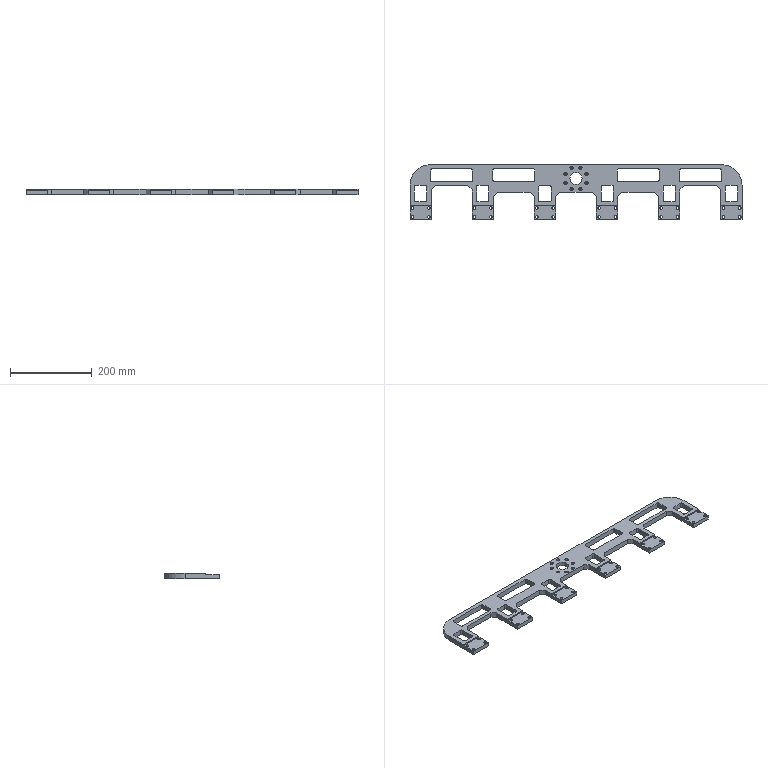NC program | NX | posted with a generic post | part box 813.6 x 134 x 13 mm
Lines 5528 to 6062 of 6062:
(PLANAR_MILL_COPY_1_COPY_1 , TOOL : D6A45)
N11006 T07 M6
N11008 G54
N11010 G17 G0 G90 X360.312 Y-40.242 S9500 M3
N11012 G43 Z30. H7
N11014 Z0.
N11016 G94 G1 Z-1. F1400.
N11018 X359.934 Y-41.05
N11020 G3 X360.8 Y-41.55 R1.
N11022 X363.15 Y-39.2 R2.35
N11024 X360.8 Y-41.55 R-2.35
N11026 X361.666 Y-41.05 R1.
N11028 G1 X361.288 Y-40.242
N11030 Z0.
N11032 G0 Z30.
N11034 X360.312 Y-62.242
N11036 Z0.
N11038 G1 Z-1.
N11040 X359.934 Y-63.05
N11042 G3 X360.8 Y-63.55 R1.
N11044 X363.15 Y-61.2 R2.35
N11046 X360.8 Y-63.55 R-2.35
N11048 X361.666 Y-63.05 R1.
N11050 G1 X361.288 Y-62.242
N11052 Z0.
N11054 G0 Z30.
N11056 X400.312
N11058 Z0.
N11060 G1 Z-1.
N11062 X399.934 Y-63.05
N11064 G3 X400.8 Y-63.55 R1.
N11066 X403.15 Y-61.2 R2.35
N11068 X400.8 Y-63.55 R-2.35
N11070 X401.666 Y-63.05 R1.
N11072 G1 X401.288 Y-62.242
N11074 Z0.
N11076 G0 Z30.
N11078 X401.842 Y-39.688
N11080 Z0.
N11082 G1 Z-1.
N11084 X402.65 Y-40.066
N11086 G3 X403.15 Y-39.2 R1.
N11088 X400.8 Y-36.85 R2.35
N11090 X403.15 Y-39.2 R-2.35
N11092 X402.65 Y-38.334 R1.
N11094 G1 X401.842 Y-38.712
N11096 Z0.
N11098 G0 Z30.
N11100 X393.7 Y-5.27
N11102 Z0.
N11104 G1 Z-1.
N11106 X394.4 Y-4.866
N11108 G3 X394.9 Y-4. R1.
N11110 G1 Y13.
N11112 G3 X392.8 Y15.1 R2.1
N11114 G1 X368.8
N11116 G3 X366.7 Y13. R2.1
N11118 G1 Y-21.
N11120 G3 X368.8 Y-23.1 R2.1
N11122 G1 X392.8
N11124 G3 X394.9 Y-21. R2.1
N11126 G1 Y-4.
N11128 G3 X394.4 Y-3.134 R1.
N11130 G1 X393.7 Y-2.73
N11132 Z0.
N11134 G0 Z30.
N11136 X306.07 Y54.9
N11138 Z0.
N11140 G1 Z-1.
N11142 X305.666 Y55.6
N11144 G3 X304.8 Y56.1 R1.
N11146 G1 X256.8
N11148 G3 X254.7 Y54. R2.1
N11150 G1 Y28.
N11152 G3 X256.8 Y25.9 R2.1
N11154 G1 X352.8
N11156 G3 X354.9 Y28. R2.1
N11158 G1 Y54.
N11160 G3 X352.8 Y56.1 R2.1
N11162 G1 X304.8
N11164 G3 X303.934 Y55.6 R1.
N11166 G1 X303.53 Y54.9
N11168 Z0.
N11170 G0 Z30.
N11172 X247.912 Y-40.242
N11174 Z0.
N11176 G1 Z-1.
N11178 X247.534 Y-41.05
N11180 G3 X248.4 Y-41.55 R1.
N11182 X250.75 Y-39.2 R2.35
N11184 X248.4 Y-41.55 R-2.35
N11186 X249.266 Y-41.05 R1.
N11188 G1 X248.888 Y-40.242
N11190 Z0.
N11192 G0 Z30.
N11194 X247.912 Y-62.242
N11196 Z0.
N11198 G1 Z-1.
N11200 X247.534 Y-63.05
N11202 G3 X248.4 Y-63.55 R1.
N11204 X250.75 Y-61.2 R2.35
N11206 X248.4 Y-63.55 R-2.35
N11208 X249.266 Y-63.05 R1.
N11210 G1 X248.888 Y-62.242
N11212 Z0.
N11214 G0 Z30.
N11216 X207.912
N11218 Z0.
N11220 G1 Z-1.
N11222 X207.534 Y-63.05
N11224 G3 X208.4 Y-63.55 R1.
N11226 X210.75 Y-61.2 R2.35
N11228 X208.4 Y-63.55 R-2.35
N11230 X209.266 Y-63.05 R1.
N11232 G1 X208.888 Y-62.242
N11234 Z0.
N11236 G0 Z30.
N11238 X207.912 Y-40.242
N11240 Z0.
N11242 G1 Z-1.
N11244 X207.534 Y-41.05
N11246 G3 X208.4 Y-41.55 R1.
N11248 X210.75 Y-39.2 R2.35
N11250 X208.4 Y-41.55 R-2.35
N11252 X209.266 Y-41.05 R1.
N11254 G1 X208.888 Y-40.242
N11256 Z0.
N11258 G0 Z30.
N11260 X215.5 Y-2.73
N11262 Z0.
N11264 G1 Z-1.
N11266 X214.8 Y-3.134
N11268 G3 X214.3 Y-4. R1.
N11270 G1 Y-21.
N11272 G3 X216.4 Y-23.1 R2.1
N11274 G1 X240.4
N11276 G3 X242.5 Y-21. R2.1
N11278 G1 Y13.
N11280 G3 X240.4 Y15.1 R2.1
N11282 G1 X216.4
N11284 G3 X214.3 Y13. R2.1
N11286 G1 Y-4.
N11288 G3 X214.8 Y-4.866 R1.
N11290 G1 X215.5 Y-5.27
N11292 Z0.
N11294 G0 Z30.
N11296 X153.67 Y54.9
N11298 Z0.
N11300 G1 Z-1.
N11302 X153.266 Y55.6
N11304 G3 X152.4 Y56.1 R1.
N11306 G1 X104.4
N11308 G3 X102.3 Y54. R2.1
N11310 G1 Y28.
N11312 G3 X104.4 Y25.9 R2.1
N11314 G1 X200.4
N11316 G3 X202.5 Y28. R2.1
N11318 G1 Y54.
N11320 G3 X200.4 Y56.1 R2.1
N11322 G1 X152.4
N11324 G3 X151.534 Y55.6 R1.
N11326 G1 X151.13 Y54.9
N11328 Z0.
N11330 G0 Z30.
N11332 X88.9 Y-5.27
N11334 Z0.
N11336 G1 Z-1.
N11338 X89.6 Y-4.866
N11340 G3 X90.1 Y-4. R1.
N11342 G1 Y13.
N11344 G3 X88. Y15.1 R2.1
N11346 G1 X64.
N11348 G3 X61.9 Y13. R2.1
N11350 G1 Y-21.
N11352 G3 X64. Y-23.1 R2.1
N11354 G1 X88.
N11356 G3 X90.1 Y-21. R2.1
N11358 G1 Y-4.
N11360 G3 X89.6 Y-3.134 R1.
N11362 G1 X88.9 Y-2.73
N11364 Z0.
N11366 G0 Z30.
N11368 X95.512 Y-40.242
N11370 Z0.
N11372 G1 Z-1.
N11374 X95.134 Y-41.05
N11376 G3 X96. Y-41.55 R1.
N11378 X98.35 Y-39.2 R2.35
N11380 X96. Y-41.55 R-2.35
N11382 X96.866 Y-41.05 R1.
N11384 G1 X96.488 Y-40.242
N11386 Z0.
N11388 G0 Z30.
N11390 X95.512 Y-62.242
N11392 Z0.
N11394 G1 Z-1.
N11396 X95.134 Y-63.05
N11398 G3 X96. Y-63.55 R1.
N11400 X98.35 Y-61.2 R2.35
N11402 X96. Y-63.55 R-2.35
N11404 X96.866 Y-63.05 R1.
N11406 G1 X96.488 Y-62.242
N11408 Z0.
N11410 G0 Z30.
N11412 X55.512
N11414 Z0.
N11416 G1 Z-1.
N11418 X55.134 Y-63.05
N11420 G3 X56. Y-63.55 R1.
N11422 X58.35 Y-61.2 R2.35
N11424 X56. Y-63.55 R-2.35
N11426 X56.866 Y-63.05 R1.
N11428 G1 X56.488 Y-62.242
N11430 Z0.
N11432 G0 Z30.
N11434 X55.512 Y-40.242
N11436 Z0.
N11438 G1 Z-1.
N11440 X55.134 Y-41.05
N11442 G3 X56. Y-41.55 R1.
N11444 X58.35 Y-39.2 R2.35
N11446 X56. Y-41.55 R-2.35
N11448 X56.866 Y-41.05 R1.
N11450 G1 X56.488 Y-40.242
N11452 Z0.
N11454 G0 Z30.
N11456 X1.287 Y62.021
N11458 Z0.
N11460 G1 Z-1.
N11462 X0.866 Y62.75
N11464 G3 X0. Y63.25 R1.
N11466 X-30.25 Y33. R30.25
N11468 X0. Y63.25 R-30.25
N11470 X-0.866 Y62.75 R1.
N11472 G1 X-1.287 Y62.021
N11474 Z0.
N11476 G0 Z30.
N11478 X-1.27 Y69.1
N11480 Z0.
N11482 G1 Z-1.
N11484 X-0.866 Y68.4
N11486 G3 X0. Y67.9 R1.
N11488 G1 X356.8
N11490 G2 X407.7 Y17. R50.9
N11492 G1 Y-66.9
N11494 G2 X406.7 Y-67.9 R1.
N11496 G1 X354.9
N11498 G2 X353.9 Y-66.9 R1.
N11500 G1 Y4.627
N11502 X344.427 Y14.1
N11504 X265.173
N11506 X255.7 Y4.627
N11508 Y-66.9
N11510 G2 X254.7 Y-67.9 R1.
N11512 G1 X202.5
N11514 G2 X201.5 Y-66.9 R1.
N11516 G1 Y-11.323
N11518 X192.027 Y-1.85
N11520 X112.773
N11522 X103.3 Y-11.323
N11524 Y-66.9
N11526 G2 X102.3 Y-67.9 R1.
N11528 G1 X50.1
N11530 G2 X49.1 Y-66.9 R1.
N11532 G1 Y-11.323
N11534 X39.627 Y-1.85
N11536 X-39.627
N11538 X-49.1 Y-11.323
N11540 Y-66.9
N11542 G2 X-50.1 Y-67.9 R1.
N11544 G1 X-102.3
N11546 G2 X-103.3 Y-66.9 R1.
N11548 G1 Y-11.323
N11550 X-112.773 Y-1.85
N11552 X-192.027
N11554 X-201.5 Y-11.323
N11556 Y-66.9
N11558 G2 X-202.5 Y-67.9 R1.
N11560 G1 X-254.7
N11562 G2 X-255.7 Y-66.9 R1.
N11564 G1 Y4.627
N11566 X-265.173 Y14.1
N11568 X-344.427
N11570 X-353.9 Y4.627
N11572 Y-66.9
N11574 G2 X-354.9 Y-67.9 R1.
N11576 G1 X-406.7
N11578 G2 X-407.7 Y-66.9 R1.
N11580 G1 Y17.
N11582 G2 X-356.8 Y67.9 R50.9
N11584 G1 X0.
N11586 G3 X0.866 Y68.4 R1.
N11588 G1 X1.27 Y69.1
N11590 Z0.
N11592 G0 Z30.
N11594 X-56.888 Y-40.242
N11596 Z0.
N11598 G1 Z-1.
N11600 X-57.266 Y-41.05
N11602 G3 X-56.4 Y-41.55 R1.
N11604 X-54.05 Y-39.2 R2.35
N11606 X-56.4 Y-41.55 R-2.35
N11608 X-55.534 Y-41.05 R1.
N11610 G1 X-55.912 Y-40.242
N11612 Z0.
N11614 G0 Z30.
N11616 X-56.888 Y-62.242
N11618 Z0.
N11620 G1 Z-1.
N11622 X-57.266 Y-63.05
N11624 G3 X-56.4 Y-63.55 R1.
N11626 X-54.05 Y-61.2 R2.35
N11628 X-56.4 Y-63.55 R-2.35
N11630 X-55.534 Y-63.05 R1.
N11632 G1 X-55.912 Y-62.242
N11634 Z0.
N11636 G0 Z30.
N11638 X-96.888
N11640 Z0.
N11642 G1 Z-1.
N11644 X-97.266 Y-63.05
N11646 G3 X-96.4 Y-63.55 R1.
N11648 X-94.05 Y-61.2 R2.35
N11650 X-96.4 Y-63.55 R-2.35
N11652 X-95.534 Y-63.05 R1.
N11654 G1 X-95.912 Y-62.242
N11656 Z0.
N11658 G0 Z30.
N11660 X-96.888 Y-40.242
N11662 Z0.
N11664 G1 Z-1.
N11666 X-97.266 Y-41.05
N11668 G3 X-96.4 Y-41.55 R1.
N11670 X-94.05 Y-39.2 R2.35
N11672 X-96.4 Y-41.55 R-2.35
N11674 X-95.534 Y-41.05 R1.
N11676 G1 X-95.912 Y-40.242
N11678 Z0.
N11680 G0 Z30.
N11682 X-89.3 Y-2.73
N11684 Z0.
N11686 G1 Z-1.
N11688 X-90. Y-3.134
N11690 G3 X-90.5 Y-4. R1.
N11692 G1 Y-21.
N11694 G3 X-88.4 Y-23.1 R2.1
N11696 G1 X-64.4
N11698 G3 X-62.3 Y-21. R2.1
N11700 G1 Y13.
N11702 G3 X-64.4 Y15.1 R2.1
N11704 G1 X-88.4
N11706 G3 X-90.5 Y13. R2.1
N11708 G1 Y-4.
N11710 G3 X-90. Y-4.866 R1.
N11712 G1 X-89.3 Y-5.27
N11714 Z0.
N11716 G0 Z30.
N11718 X-151.13 Y54.9
N11720 Z0.
N11722 G1 Z-1.
N11724 X-151.534 Y55.6
N11726 G3 X-152.4 Y56.1 R1.
N11728 G1 X-200.4
N11730 G3 X-202.5 Y54. R2.1
N11732 G1 Y28.
N11734 G3 X-200.4 Y25.9 R2.1
N11736 G1 X-104.4
N11738 G3 X-102.3 Y28. R2.1
N11740 G1 Y54.
N11742 G3 X-104.4 Y56.1 R2.1
N11744 G1 X-152.4
N11746 G3 X-153.266 Y55.6 R1.
N11748 G1 X-153.67 Y54.9
N11750 Z0.
N11752 G0 Z30.
N11754 X-209.288 Y-40.242
N11756 Z0.
N11758 G1 Z-1.
N11760 X-209.666 Y-41.05
N11762 G3 X-208.8 Y-41.55 R1.
N11764 X-206.45 Y-39.2 R2.35
N11766 X-208.8 Y-41.55 R-2.35
N11768 X-207.934 Y-41.05 R1.
N11770 G1 X-208.312 Y-40.242
N11772 Z0.
N11774 G0 Z30.
N11776 X-209.288 Y-62.242
N11778 Z0.
N11780 G1 Z-1.
N11782 X-209.666 Y-63.05
N11784 G3 X-208.8 Y-63.55 R1.
N11786 X-206.45 Y-61.2 R2.35
N11788 X-208.8 Y-63.55 R-2.35
N11790 X-207.934 Y-63.05 R1.
N11792 G1 X-208.312 Y-62.242
N11794 Z0.
N11796 G0 Z30.
N11798 X-249.288
N11800 Z0.
N11802 G1 Z-1.
N11804 X-249.666 Y-63.05
N11806 G3 X-248.8 Y-63.55 R1.
N11808 X-246.45 Y-61.2 R2.35
N11810 X-248.8 Y-63.55 R-2.35
N11812 X-247.934 Y-63.05 R1.
N11814 G1 X-248.312 Y-62.242
N11816 Z0.
N11818 G0 Z30.
N11820 X-249.288 Y-40.242
N11822 Z0.
N11824 G1 Z-1.
N11826 X-249.666 Y-41.05
N11828 G3 X-248.8 Y-41.55 R1.
N11830 X-246.45 Y-39.2 R2.35
N11832 X-248.8 Y-41.55 R-2.35
N11834 X-247.934 Y-41.05 R1.
N11836 G1 X-248.312 Y-40.242
N11838 Z0.
N11840 G0 Z30.
N11842 X-241.7 Y-2.73
N11844 Z0.
N11846 G1 Z-1.
N11848 X-242.4 Y-3.134
N11850 G3 X-242.9 Y-4. R1.
N11852 G1 Y-21.
N11854 G3 X-240.8 Y-23.1 R2.1
N11856 G1 X-216.8
N11858 G3 X-214.7 Y-21. R2.1
N11860 G1 Y13.
N11862 G3 X-216.8 Y15.1 R2.1
N11864 G1 X-240.8
N11866 G3 X-242.9 Y13. R2.1
N11868 G1 Y-4.
N11870 G3 X-242.4 Y-4.866 R1.
N11872 G1 X-241.7 Y-5.27
N11874 Z0.
N11876 G0 Z30.
N11878 X-303.53 Y54.9
N11880 Z0.
N11882 G1 Z-1.
N11884 X-303.934 Y55.6
N11886 G3 X-304.8 Y56.1 R1.
N11888 G1 X-352.8
N11890 G3 X-354.9 Y54. R2.1
N11892 G1 Y28.
N11894 G3 X-352.8 Y25.9 R2.1
N11896 G1 X-256.8
N11898 G3 X-254.7 Y28. R2.1
N11900 G1 Y54.
N11902 G3 X-256.8 Y56.1 R2.1
N11904 G1 X-304.8
N11906 G3 X-305.666 Y55.6 R1.
N11908 G1 X-306.07 Y54.9
N11910 Z0.
N11912 G0 Z30.
N11914 X-394.1 Y-2.73
N11916 Z0.
N11918 G1 Z-1.
N11920 X-394.8 Y-3.134
N11922 G3 X-395.3 Y-4. R1.
N11924 G1 Y-21.
N11926 G3 X-393.2 Y-23.1 R2.1
N11928 G1 X-369.2
N11930 G3 X-367.1 Y-21. R2.1
N11932 G1 Y13.
N11934 G3 X-369.2 Y15.1 R2.1
N11936 G1 X-393.2
N11938 G3 X-395.3 Y13. R2.1
N11940 G1 Y-4.
N11942 G3 X-394.8 Y-4.866 R1.
N11944 G1 X-394.1 Y-5.27
N11946 Z0.
N11948 G0 Z30.
N11950 X-402.242 Y-38.712
N11952 Z0.
N11954 G1 Z-1.
N11956 X-403.05 Y-38.334
N11958 G3 X-403.55 Y-39.2 R1.
N11960 X-401.2 Y-41.55 R2.35
N11962 X-403.55 Y-39.2 R-2.35
N11964 X-403.05 Y-40.066 R1.
N11966 G1 X-402.242 Y-39.688
N11968 Z0.
N11970 G0 Z30.
N11972 Y-60.712
N11974 Z0.
N11976 G1 Z-1.
N11978 X-403.05 Y-60.334
N11980 G3 X-403.55 Y-61.2 R1.
N11982 X-401.2 Y-63.55 R2.35
N11984 X-403.55 Y-61.2 R-2.35
N11986 X-403.05 Y-62.066 R1.
N11988 G1 X-402.242 Y-61.688
N11990 Z0.
N11992 G0 Z30.
N11994 X-361.688 Y-62.242
N11996 Z0.
N11998 G1 Z-1.
N12000 X-362.066 Y-63.05
N12002 G3 X-361.2 Y-63.55 R1.
N12004 X-358.85 Y-61.2 R2.35
N12006 X-361.2 Y-63.55 R-2.35
N12008 X-360.334 Y-63.05 R1.
N12010 G1 X-360.712 Y-62.242
N12012 Z0.
N12014 G0 Z30.
N12016 X-361.688 Y-40.242
N12018 Z0.
N12020 G1 Z-1.
N12022 X-362.066 Y-41.05
N12024 G3 X-361.2 Y-41.55 R1.
N12026 X-358.85 Y-39.2 R2.35
N12028 X-361.2 Y-41.55 R-2.35
N12030 X-360.334 Y-41.05 R1.
N12032 G1 X-360.712 Y-40.242
N12034 Z0.
N12036 G0 Z30.
(PLANAR_MILL_COPY_1_COPY_1_COPY , TOOL : D6A45)
N12038 X-12.833 Y34.309
N12040 Z-3.
N12042 G1 Z-4.
N12044 X-13.6 Y33.866
N12046 G3 X-14.1 Y33. R1.
N12048 X0. Y18.9 R14.1
N12050 X-14.1 Y33. R-14.1
N12052 X-13.6 Y32.134 R1.
N12054 G1 X-12.833 Y31.691
N12056 Z-3.
N12058 G0 Z30.
N12060 M5
N12062 M2